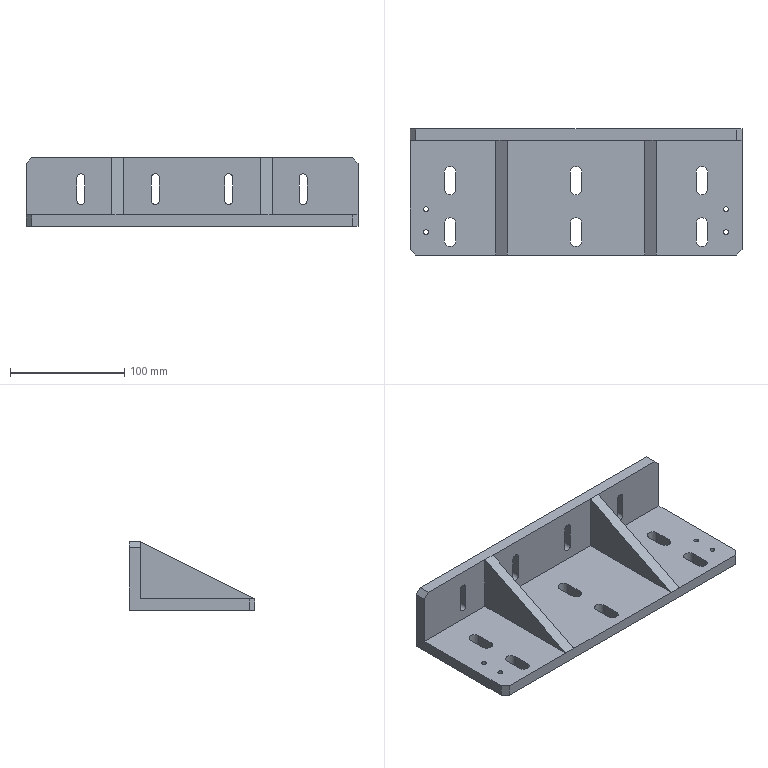Part | NX | features BREP 1 | 1 solid | 74 faces | box 290 x 110 x 60 mm | volume 492094 mm3 | plane 42 | cylinder 32 | commonest cylinder face diameters 7 x12 10 x12 4.2 x8